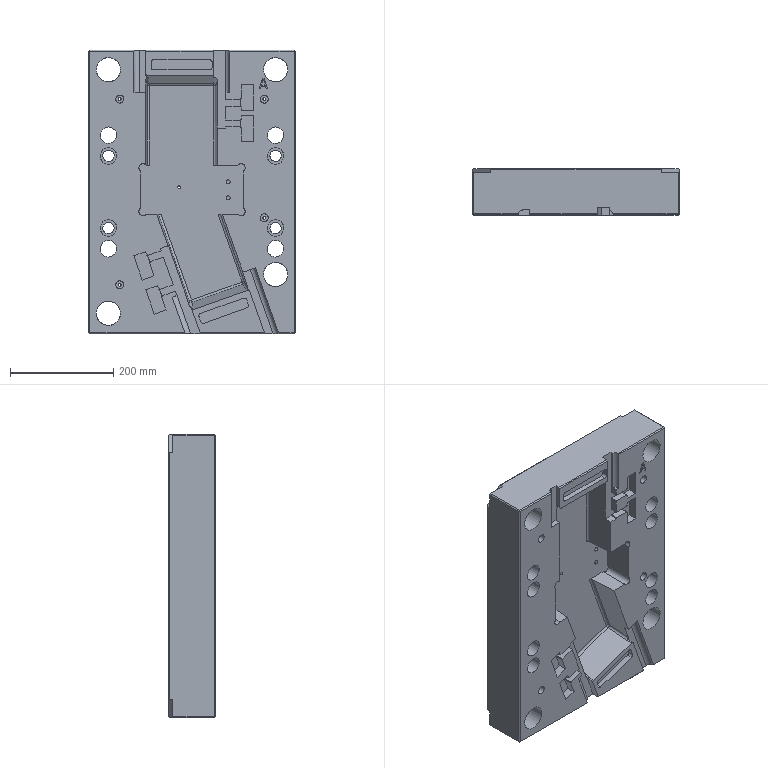Part | STEP file | A-PLATE_id546_x_t | 1 solid | 248 faces | box 400 x 90 x 550 mm | volume 14561004 mm3 | plane 161 | cylinder 70 | cone 10 | other 5 | spline 2 | commonest cylinder face diameters 10 x25 32 x8 5.5 x4 8 x4 15.681 x4 16 x4